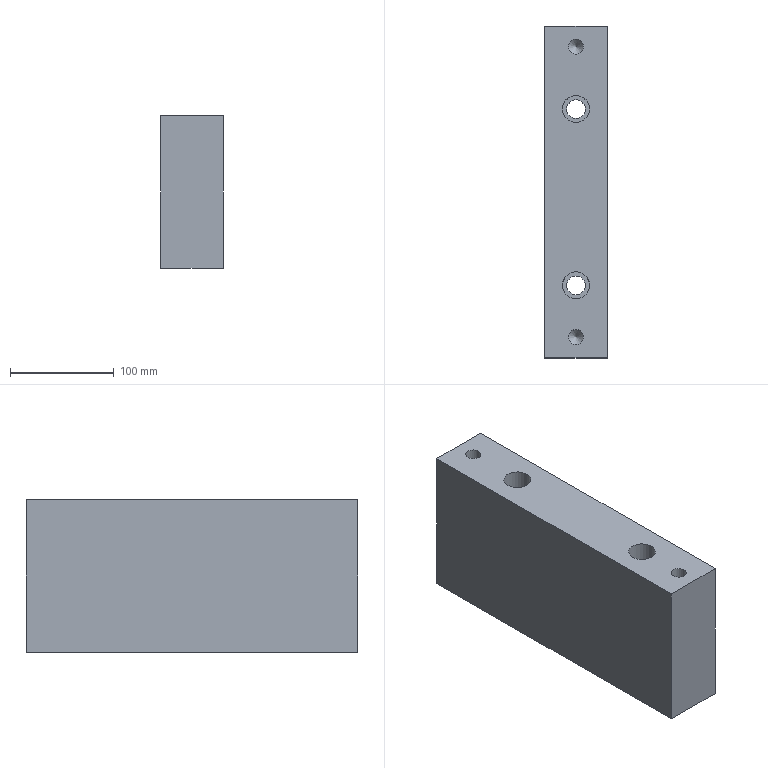Part | STEP file | lll_id1782_x_t | 1 solid | 16 faces | box 60 x 320 x 147.5 mm | volume 2706247 mm3 | plane 8 | cylinder 6 | cone 2 | commonest cylinder face diameters 14.506 x2 18.009 x2 26.008 x2
STEP:
#1=CARTESIAN_POINT('',(210.439,350.,370.));
#2=VERTEX_POINT('',#1);
#3=CARTESIAN_POINT('',(197.435,350.,370.));
#4=DIRECTION('',(0.,0.,1.));
#5=DIRECTION('',(1.,0.,0.));
#6=AXIS2_PLACEMENT_3D('',#3,#4,#5);
#7=CIRCLE('',#6,13.004);
#8=EDGE_CURVE('',#2,#2,#7,.T.);
#9=ORIENTED_EDGE('',*,*,#8,.F.);
#10=EDGE_LOOP('',(#9));
#11=FACE_BOUND('',#10,.T.);
#12=CARTESIAN_POINT('',(210.439,520.,370.));
#13=VERTEX_POINT('',#12);
#14=CARTESIAN_POINT('',(197.435,520.,370.));
#15=DIRECTION('',(0.,0.,1.));
#16=DIRECTION('',(1.,0.,0.));
#17=AXIS2_PLACEMENT_3D('',#14,#15,#16);
#18=CIRCLE('',#17,13.004);
#19=EDGE_CURVE('',#13,#13,#18,.T.);
#20=ORIENTED_EDGE('',*,*,#19,.F.);
#21=EDGE_LOOP('',(#20));
#22=FACE_BOUND('',#21,.T.);
#23=CARTESIAN_POINT('',(167.435,600.,370.));
#24=VERTEX_POINT('',#23);
#25=CARTESIAN_POINT('',(167.435,280.,370.));
#26=VERTEX_POINT('',#25);
#27=CARTESIAN_POINT('',(167.435,600.,370.));
#28=DIRECTION('',(0.,-1.,0.));
#29=VECTOR('',#28,1.);
#30=LINE('',#27,#29);
#31=EDGE_CURVE('',#24,#26,#30,.T.);
#32=ORIENTED_EDGE('',*,*,#31,.T.);
#33=CARTESIAN_POINT('',(227.435,280.,370.));
#34=VERTEX_POINT('',#33);
#35=CARTESIAN_POINT('',(-2018.88,280.,370.));
#36=DIRECTION('',(1.,0.,0.));
#37=VECTOR('',#36,1.);
#38=LINE('',#35,#37);
#39=EDGE_CURVE('',#26,#34,#38,.T.);
#40=ORIENTED_EDGE('',*,*,#39,.T.);
#41=CARTESIAN_POINT('',(227.435,600.,370.));
#42=VERTEX_POINT('',#41);
#43=CARTESIAN_POINT('',(227.435,0.9999,370.));
#44=DIRECTION('',(0.,1.,0.));
#45=VECTOR('',#44,1.);
#46=LINE('',#43,#45);
#47=EDGE_CURVE('',#34,#42,#46,.T.);
#48=ORIENTED_EDGE('',*,*,#47,.T.);
#49=CARTESIAN_POINT('',(4137.435,600.,370.));
#50=DIRECTION('',(-1.,0.,0.));
#51=VECTOR('',#50,1.);
#52=LINE('',#49,#51);
#53=EDGE_CURVE('',#42,#24,#52,.T.);
#54=ORIENTED_EDGE('',*,*,#53,.T.);
#55=EDGE_LOOP('',(#32,#40,#48,#54));
#56=FACE_BOUND('',#55,.T.);
#57=CARTESIAN_POINT('',(204.688,580.,370.));
#58=VERTEX_POINT('',#57);
#59=CARTESIAN_POINT('',(197.435,580.,370.));
#60=DIRECTION('',(0.,0.,-1.));
#61=DIRECTION('',(1.,0.,0.));
#62=AXIS2_PLACEMENT_3D('',#59,#60,#61);
#63=CIRCLE('',#62,7.253);
#64=EDGE_CURVE('',#58,#58,#63,.T.);
#65=ORIENTED_EDGE('',*,*,#64,.T.);
#66=EDGE_LOOP('',(#65));
#67=FACE_BOUND('',#66,.T.);
#68=CARTESIAN_POINT('',(204.688,300.,370.));
#69=VERTEX_POINT('',#68);
#70=CARTESIAN_POINT('',(197.435,300.,370.));
#71=DIRECTION('',(0.,0.,1.));
#72=DIRECTION('',(1.,0.,0.));
#73=AXIS2_PLACEMENT_3D('',#70,#71,#72);
#74=CIRCLE('',#73,7.253);
#75=EDGE_CURVE('',#69,#69,#74,.T.);
#76=ORIENTED_EDGE('',*,*,#75,.F.);
#77=EDGE_LOOP('',(#76));
#78=FACE_BOUND('',#77,.T.);
#79=CARTESIAN_POINT('',(-2018.88,0.9999,370.));
#80=DIRECTION('',(0.,0.,-1.));
#81=DIRECTION('',(1.,0.,0.));
#82=AXIS2_PLACEMENT_3D('',#79,#80,#81);
#83=PLANE('',#82);
#84=ADVANCED_FACE('',(#11,#22,#56,#67,#78),#83,.F.);
#85=CARTESIAN_POINT('',(227.435,280.,222.5));
#86=VERTEX_POINT('',#85);
#87=CARTESIAN_POINT('',(167.435,280.,222.5));
#88=VERTEX_POINT('',#87);
#89=CARTESIAN_POINT('',(-2018.88,280.,222.5));
#90=DIRECTION('',(-1.,0.,0.));
#91=VECTOR('',#90,1.);
#92=LINE('',#89,#91);
#93=EDGE_CURVE('',#86,#88,#92,.T.);
#94=ORIENTED_EDGE('',*,*,#93,.T.);
#95=CARTESIAN_POINT('',(167.435,600.,222.5));
#96=VERTEX_POINT('',#95);
#97=CARTESIAN_POINT('',(167.435,600.,222.5));
#98=DIRECTION('',(0.,-1.,0.));
#99=VECTOR('',#98,1.);
#100=LINE('',#97,#99);
#101=EDGE_CURVE('',#96,#88,#100,.T.);
#102=ORIENTED_EDGE('',*,*,#101,.F.);
#103=CARTESIAN_POINT('',(227.435,600.,222.5));
#104=VERTEX_POINT('',#103);
#105=CARTESIAN_POINT('',(4137.435,600.,222.5));
#106=DIRECTION('',(-1.,0.,0.));
#107=VECTOR('',#106,1.);
#108=LINE('',#105,#107);
#109=EDGE_CURVE('',#104,#96,#108,.T.);
#110=ORIENTED_EDGE('',*,*,#109,.F.);
#111=CARTESIAN_POINT('',(227.435,0.9999,222.5));
#112=DIRECTION('',(0.,-1.,0.));
#113=VECTOR('',#112,1.);
#114=LINE('',#111,#113);
#115=EDGE_CURVE('',#104,#86,#114,.T.);
#116=ORIENTED_EDGE('',*,*,#115,.T.);
#117=EDGE_LOOP('',(#94,#102,#110,#116));
#118=FACE_BOUND('',#117,.T.);
#119=CARTESIAN_POINT('',(206.44,520.,222.5));
#120=VERTEX_POINT('',#119);
#121=CARTESIAN_POINT('',(197.435,520.,222.5));
#122=DIRECTION('',(0.,0.,-1.));
#123=DIRECTION('',(1.,0.,0.));
#124=AXIS2_PLACEMENT_3D('',#121,#122,#123);
#125=CIRCLE('',#124,9.005);
#126=EDGE_CURVE('',#120,#120,#125,.T.);
#127=ORIENTED_EDGE('',*,*,#126,.F.);
#128=EDGE_LOOP('',(#127));
#129=FACE_BOUND('',#128,.T.);
#130=CARTESIAN_POINT('',(206.44,350.,222.5));
#131=VERTEX_POINT('',#130);
#132=CARTESIAN_POINT('',(197.435,350.,222.5));
#133=DIRECTION('',(0.,0.,-1.));
#134=DIRECTION('',(1.,0.,0.));
#135=AXIS2_PLACEMENT_3D('',#132,#133,#134);
#136=CIRCLE('',#135,9.005);
#137=EDGE_CURVE('',#131,#131,#136,.T.);
#138=ORIENTED_EDGE('',*,*,#137,.F.);
#139=EDGE_LOOP('',(#138));
#140=FACE_BOUND('',#139,.T.);
#141=CARTESIAN_POINT('',(-2018.88,0.9999,222.5));
#142=DIRECTION('',(0.,0.,-1.));
#143=DIRECTION('',(1.,0.,0.));
#144=AXIS2_PLACEMENT_3D('',#141,#142,#143);
#145=PLANE('',#144);
#146=ADVANCED_FACE('',(#118,#129,#140),#145,.T.);
#147=CARTESIAN_POINT('',(167.435,280.,360.));
#148=DIRECTION('',(0.,0.,-1.));
#149=VECTOR('',#148,1.);
#150=LINE('',#147,#149);
#151=EDGE_CURVE('',#26,#88,#150,.T.);
#152=ORIENTED_EDGE('',*,*,#151,.F.);
#153=ORIENTED_EDGE('',*,*,#31,.F.);
#154=CARTESIAN_POINT('',(167.435,600.,360.));
#155=DIRECTION('',(0.,0.,-1.));
#156=VECTOR('',#155,1.);
#157=LINE('',#154,#156);
#158=EDGE_CURVE('',#24,#96,#157,.T.);
#159=ORIENTED_EDGE('',*,*,#158,.T.);
#160=ORIENTED_EDGE('',*,*,#101,.T.);
#161=EDGE_LOOP('',(#152,#153,#159,#160));
#162=FACE_OUTER_BOUND('',#161,.T.);
#163=CARTESIAN_POINT('',(167.435,600.,360.));
#164=DIRECTION('',(-1.,0.,0.));
#165=DIRECTION('',(0.,0.,-1.));
#166=AXIS2_PLACEMENT_3D('',#163,#164,#165);
#167=PLANE('',#166);
#168=ADVANCED_FACE('',(#162),#167,.T.);
#169=ORIENTED_EDGE('',*,*,#47,.F.);
#170=CARTESIAN_POINT('',(227.435,280.,291.25));
#171=DIRECTION('',(0.,0.,1.));
#172=VECTOR('',#171,1.);
#173=LINE('',#170,#172);
#174=EDGE_CURVE('',#86,#34,#173,.T.);
#175=ORIENTED_EDGE('',*,*,#174,.F.);
#176=ORIENTED_EDGE('',*,*,#115,.F.);
#177=CARTESIAN_POINT('',(227.435,600.,360.));
#178=DIRECTION('',(0.,0.,1.));
#179=VECTOR('',#178,1.);
#180=LINE('',#177,#179);
#181=EDGE_CURVE('',#104,#42,#180,.T.);
#182=ORIENTED_EDGE('',*,*,#181,.T.);
#183=EDGE_LOOP('',(#169,#175,#176,#182));
#184=FACE_OUTER_BOUND('',#183,.T.);
#185=CARTESIAN_POINT('',(227.435,-0.00005,291.25));
#186=DIRECTION('',(-1.,0.,0.));
#187=DIRECTION('',(0.,0.,-1.));
#188=AXIS2_PLACEMENT_3D('',#185,#186,#187);
#189=PLANE('',#188);
#190=ADVANCED_FACE('',(#184),#189,.F.);
#191=ORIENTED_EDGE('',*,*,#181,.F.);
#192=ORIENTED_EDGE('',*,*,#109,.T.);
#193=ORIENTED_EDGE('',*,*,#158,.F.);
#194=ORIENTED_EDGE('',*,*,#53,.F.);
#195=EDGE_LOOP('',(#191,#192,#193,#194));
#196=FACE_OUTER_BOUND('',#195,.T.);
#197=CARTESIAN_POINT('',(4137.435,600.,360.));
#198=DIRECTION('',(0.,1.,0.));
#199=DIRECTION('',(0.,0.,1.));
#200=AXIS2_PLACEMENT_3D('',#197,#198,#199);
#201=PLANE('',#200);
#202=ADVANCED_FACE('',(#196),#201,.T.);
#203=CARTESIAN_POINT('',(188.431,520.,302.5));
#204=VERTEX_POINT('',#203);
#205=CARTESIAN_POINT('',(197.435,520.,302.5));
#206=DIRECTION('',(0.,0.,1.));
#207=DIRECTION('',(-1.,0.,0.));
#208=AXIS2_PLACEMENT_3D('',#205,#206,#207);
#209=CIRCLE('',#208,9.005);
#210=EDGE_CURVE('',#204,#204,#209,.T.);
#211=ORIENTED_EDGE('',*,*,#210,.T.);
#212=EDGE_LOOP('',(#211));
#213=FACE_BOUND('',#212,.T.);
#214=ORIENTED_EDGE('',*,*,#126,.T.);
#215=EDGE_LOOP('',(#214));
#216=FACE_BOUND('',#215,.T.);
#217=CARTESIAN_POINT('',(197.435,520.,420.));
#218=DIRECTION('',(0.,0.,-1.));
#219=DIRECTION('',(1.,0.,0.));
#220=AXIS2_PLACEMENT_3D('',#217,#218,#219);
#221=CYLINDRICAL_SURFACE('',#220,9.005);
#222=ADVANCED_FACE('',(#213,#216),#221,.F.);
#223=ORIENTED_EDGE('',*,*,#210,.F.);
#224=EDGE_LOOP('',(#223));
#225=FACE_BOUND('',#224,.T.);
#226=CARTESIAN_POINT('',(210.439,520.,302.5));
#227=VERTEX_POINT('',#226);
#228=CARTESIAN_POINT('',(197.435,520.,302.5));
#229=DIRECTION('',(0.,0.,1.));
#230=DIRECTION('',(-1.,0.,0.));
#231=AXIS2_PLACEMENT_3D('',#228,#229,#230);
#232=CIRCLE('',#231,13.004);
#233=EDGE_CURVE('',#227,#227,#232,.T.);
#234=ORIENTED_EDGE('',*,*,#233,.T.);
#235=EDGE_LOOP('',(#234));
#236=FACE_BOUND('',#235,.T.);
#237=CARTESIAN_POINT('',(197.435,520.,302.5));
#238=DIRECTION('',(0.,0.,-1.));
#239=DIRECTION('',(-1.,0.,0.));
#240=AXIS2_PLACEMENT_3D('',#237,#238,#239);
#241=PLANE('',#240);
#242=ADVANCED_FACE('',(#225,#236),#241,.F.);
#243=ORIENTED_EDGE('',*,*,#233,.F.);
#244=EDGE_LOOP('',(#243));
#245=FACE_BOUND('',#244,.T.);
#246=ORIENTED_EDGE('',*,*,#19,.T.);
#247=EDGE_LOOP('',(#246));
#248=FACE_BOUND('',#247,.T.);
#249=CARTESIAN_POINT('',(197.435,520.,420.));
#250=DIRECTION('',(0.,0.,-1.));
#251=DIRECTION('',(1.,0.,0.));
#252=AXIS2_PLACEMENT_3D('',#249,#250,#251);
#253=CYLINDRICAL_SURFACE('',#252,13.004);
#254=ADVANCED_FACE('',(#245,#248),#253,.F.);
#255=CARTESIAN_POINT('',(188.431,350.,302.5));
#256=VERTEX_POINT('',#255);
#257=CARTESIAN_POINT('',(197.435,350.,302.5));
#258=DIRECTION('',(0.,0.,1.));
#259=DIRECTION('',(-1.,0.,0.));
#260=AXIS2_PLACEMENT_3D('',#257,#258,#259);
#261=CIRCLE('',#260,9.005);
#262=EDGE_CURVE('',#256,#256,#261,.T.);
#263=ORIENTED_EDGE('',*,*,#262,.T.);
#264=EDGE_LOOP('',(#263));
#265=FACE_BOUND('',#264,.T.);
#266=ORIENTED_EDGE('',*,*,#137,.T.);
#267=EDGE_LOOP('',(#266));
#268=FACE_BOUND('',#267,.T.);
#269=CARTESIAN_POINT('',(197.435,350.,420.));
#270=DIRECTION('',(0.,0.,-1.));
#271=DIRECTION('',(1.,0.,0.));
#272=AXIS2_PLACEMENT_3D('',#269,#270,#271);
#273=CYLINDRICAL_SURFACE('',#272,9.005);
#274=ADVANCED_FACE('',(#265,#268),#273,.F.);
#275=ORIENTED_EDGE('',*,*,#262,.F.);
#276=EDGE_LOOP('',(#275));
#277=FACE_BOUND('',#276,.T.);
#278=CARTESIAN_POINT('',(210.439,350.,302.5));
#279=VERTEX_POINT('',#278);
#280=CARTESIAN_POINT('',(197.435,350.,302.5));
#281=DIRECTION('',(0.,0.,1.));
#282=DIRECTION('',(1.,0.,0.));
#283=AXIS2_PLACEMENT_3D('',#280,#281,#282);
#284=CIRCLE('',#283,13.004);
#285=EDGE_CURVE('',#279,#279,#284,.T.);
#286=ORIENTED_EDGE('',*,*,#285,.T.);
#287=EDGE_LOOP('',(#286));
#288=FACE_BOUND('',#287,.T.);
#289=CARTESIAN_POINT('',(197.435,350.,302.5));
#290=DIRECTION('',(0.,0.,-1.));
#291=DIRECTION('',(-1.,0.,0.));
#292=AXIS2_PLACEMENT_3D('',#289,#290,#291);
#293=PLANE('',#292);
#294=ADVANCED_FACE('',(#277,#288),#293,.F.);
#295=ORIENTED_EDGE('',*,*,#285,.F.);
#296=EDGE_LOOP('',(#295));
#297=FACE_BOUND('',#296,.T.);
#298=ORIENTED_EDGE('',*,*,#8,.T.);
#299=EDGE_LOOP('',(#298));
#300=FACE_BOUND('',#299,.T.);
#301=CARTESIAN_POINT('',(197.435,350.,420.));
#302=DIRECTION('',(0.,0.,-1.));
#303=DIRECTION('',(1.,0.,0.));
#304=AXIS2_PLACEMENT_3D('',#301,#302,#303);
#305=CYLINDRICAL_SURFACE('',#304,13.004);
#306=ADVANCED_FACE('',(#297,#300),#305,.F.);
#307=ORIENTED_EDGE('',*,*,#151,.T.);
#308=ORIENTED_EDGE('',*,*,#93,.F.);
#309=ORIENTED_EDGE('',*,*,#174,.T.);
#310=ORIENTED_EDGE('',*,*,#39,.F.);
#311=EDGE_LOOP('',(#307,#308,#309,#310));
#312=FACE_OUTER_BOUND('',#311,.T.);
#313=CARTESIAN_POINT('',(197.435,280.,321.25));
#314=DIRECTION('',(0.,1.,0.));
#315=DIRECTION('',(0.,0.,1.));
#316=AXIS2_PLACEMENT_3D('',#313,#314,#315);
#317=PLANE('',#316);
#318=ADVANCED_FACE('',(#312),#317,.F.);
#319=CARTESIAN_POINT('',(190.182,580.,332.247));
#320=VERTEX_POINT('',#319);
#321=CARTESIAN_POINT('',(197.435,580.,332.247));
#322=DIRECTION('',(0.,0.,-1.));
#323=DIRECTION('',(-1.,0.,0.));
#324=AXIS2_PLACEMENT_3D('',#321,#322,#323);
#325=CIRCLE('',#324,7.253);
#326=EDGE_CURVE('',#320,#320,#325,.T.);
#327=ORIENTED_EDGE('',*,*,#326,.T.);
#328=EDGE_LOOP('',(#327));
#329=FACE_BOUND('',#328,.T.);
#330=ORIENTED_EDGE('',*,*,#64,.F.);
#331=EDGE_LOOP('',(#330));
#332=FACE_BOUND('',#331,.T.);
#333=CARTESIAN_POINT('',(197.435,580.,370.));
#334=DIRECTION('',(0.,0.,-1.));
#335=DIRECTION('',(1.,0.,0.));
#336=AXIS2_PLACEMENT_3D('',#333,#334,#335);
#337=CYLINDRICAL_SURFACE('',#336,7.253);
#338=ADVANCED_FACE('',(#329,#332),#337,.F.);
#339=CARTESIAN_POINT('',(197.435,580.,324.994));
#340=VERTEX_POINT('',#339);
#341=VERTEX_LOOP('',#340);
#342=FACE_BOUND('',#341,.T.);
#343=ORIENTED_EDGE('',*,*,#326,.F.);
#344=EDGE_LOOP('',(#343));
#345=FACE_BOUND('',#344,.T.);
#346=CARTESIAN_POINT('',(197.435,580.,332.247));
#347=DIRECTION('',(0.,0.,1.));
#348=DIRECTION('',(1.,0.,0.));
#349=AXIS2_PLACEMENT_3D('',#346,#347,#348);
#350=CONICAL_SURFACE('',#349,7.253,45.);
#351=ADVANCED_FACE('',(#342,#345),#350,.F.);
#352=CARTESIAN_POINT('',(190.182,300.,332.247));
#353=VERTEX_POINT('',#352);
#354=CARTESIAN_POINT('',(197.435,300.,332.247));
#355=DIRECTION('',(0.,0.,1.));
#356=DIRECTION('',(-1.,0.,0.));
#357=AXIS2_PLACEMENT_3D('',#354,#355,#356);
#358=CIRCLE('',#357,7.253);
#359=EDGE_CURVE('',#353,#353,#358,.T.);
#360=ORIENTED_EDGE('',*,*,#359,.F.);
#361=EDGE_LOOP('',(#360));
#362=FACE_BOUND('',#361,.T.);
#363=ORIENTED_EDGE('',*,*,#75,.T.);
#364=EDGE_LOOP('',(#363));
#365=FACE_BOUND('',#364,.T.);
#366=CARTESIAN_POINT('',(197.435,300.,370.));
#367=DIRECTION('',(0.,0.,-1.));
#368=DIRECTION('',(1.,0.,0.));
#369=AXIS2_PLACEMENT_3D('',#366,#367,#368);
#370=CYLINDRICAL_SURFACE('',#369,7.253);
#371=ADVANCED_FACE('',(#362,#365),#370,.F.);
#372=CARTESIAN_POINT('',(197.435,300.,324.994));
#373=VERTEX_POINT('',#372);
#374=VERTEX_LOOP('',#373);
#375=FACE_BOUND('',#374,.T.);
#376=ORIENTED_EDGE('',*,*,#359,.T.);
#377=EDGE_LOOP('',(#376));
#378=FACE_BOUND('',#377,.T.);
#379=CARTESIAN_POINT('',(197.435,300.,332.247));
#380=DIRECTION('',(0.,0.,1.));
#381=DIRECTION('',(1.,0.,0.));
#382=AXIS2_PLACEMENT_3D('',#379,#380,#381);
#383=CONICAL_SURFACE('',#382,7.253,45.);
#384=ADVANCED_FACE('',(#375,#378),#383,.F.);
#385=CLOSED_SHELL('',(#84,#146,#168,#190,#202,#222,#242,#254,#274,#294,#306,#318,#338,#351,#371,#384));
#386=MANIFOLD_SOLID_BREP('',#385);
#387=(LENGTH_UNIT()NAMED_UNIT(*)SI_UNIT(.MILLI.,.METRE.));
#388=UNCERTAINTY_MEASURE_WITH_UNIT(LENGTH_MEASURE(0.00002),#387,'','');
#389=(NAMED_UNIT(*)PLANE_ANGLE_UNIT()SI_UNIT($,.RADIAN.));
#390=PLANE_ANGLE_MEASURE_WITH_UNIT(PLANE_ANGLE_MEASURE(0.01745),#389);
#391=DIMENSIONAL_EXPONENTS(0.,0.,0.,0.,0.,0.,0.);
#392=(CONVERSION_BASED_UNIT('DEGREE',#390)NAMED_UNIT(#391)PLANE_ANGLE_UNIT());
#393=(NAMED_UNIT(*)SI_UNIT($,.STERADIAN.)SOLID_ANGLE_UNIT());
#394=(GEOMETRIC_REPRESENTATION_CONTEXT(3)GLOBAL_UNCERTAINTY_ASSIGNED_CONTEXT((#388))GLOBAL_UNIT_ASSIGNED_CONTEXT((#387,#392,#393))REPRESENTATION_CONTEXT('',''));
#395=ADVANCED_BREP_SHAPE_REPRESENTATION('',(#386),#394);